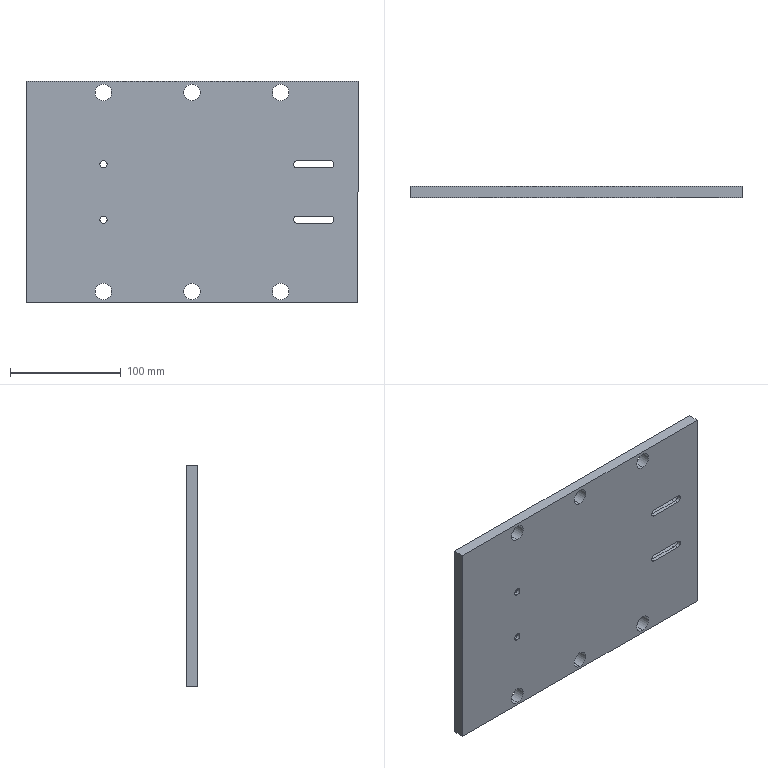Part | SolidWorks | features ICE 3, Extrusion 1, HoleWzd 1, LPattern 1 | 1 solid | 46 faces | box 300 x 10 x 200 mm | volume 580619 mm3 | cylinder 28 | plane 18 | commonest cylinder face diameters 15 x12 6.6 x8 11 x8
STEP:
#1=CARTESIAN_POINT('',(-80.,-1.8,-30.5));
#2=VERTEX_POINT('',#1);
#3=CARTESIAN_POINT('',(-80.,-1.8,-19.5));
#4=VERTEX_POINT('',#3);
#5=CARTESIAN_POINT('',(-80.,-1.8,-25.));
#6=DIRECTION('',(0.,1.,0.));
#7=DIRECTION('',(0.,0.,1.));
#8=AXIS2_PLACEMENT_3D('',#5,#6,#7);
#9=CIRCLE('',#8,5.5);
#10=EDGE_CURVE('',#2,#4,#9,.T.);
#11=ORIENTED_EDGE('',*,*,#10,.F.);
#12=CARTESIAN_POINT('',(-80.,5.,-30.5));
#13=VERTEX_POINT('',#12);
#14=CARTESIAN_POINT('',(-80.,5.,-30.5));
#15=DIRECTION('',(0.,1.,0.));
#16=VECTOR('',#15,1000.);
#17=LINE('',#14,#16);
#18=EDGE_CURVE('',#2,#13,#17,.T.);
#19=ORIENTED_EDGE('',*,*,#18,.T.);
#20=CARTESIAN_POINT('',(-80.,5.,-19.5));
#21=VERTEX_POINT('',#20);
#22=CARTESIAN_POINT('',(-80.,5.,-25.));
#23=DIRECTION('',(0.,1.,0.));
#24=DIRECTION('',(0.,0.,1.));
#25=AXIS2_PLACEMENT_3D('',#22,#23,#24);
#26=CIRCLE('',#25,5.5);
#27=EDGE_CURVE('',#13,#21,#26,.T.);
#28=ORIENTED_EDGE('',*,*,#27,.T.);
#29=CARTESIAN_POINT('',(-80.,5.,-19.5));
#30=DIRECTION('',(0.,1.,0.));
#31=VECTOR('',#30,1000.);
#32=LINE('',#29,#31);
#33=EDGE_CURVE('',#4,#21,#32,.T.);
#34=ORIENTED_EDGE('',*,*,#33,.F.);
#35=EDGE_LOOP('',(#11,#19,#28,#34));
#36=FACE_OUTER_BOUND('',#35,.T.);
#37=CARTESIAN_POINT('',(-80.,5.,-25.));
#38=DIRECTION('',(0.,1.,0.));
#39=DIRECTION('',(0.,0.,1.));
#40=AXIS2_PLACEMENT_3D('',#37,#38,#39);
#41=CYLINDRICAL_SURFACE('',#40,5.5);
#42=ADVANCED_FACE('',(#36),#41,.F.);
#43=CARTESIAN_POINT('',(-80.,-5.,-28.3));
#44=VERTEX_POINT('',#43);
#45=CARTESIAN_POINT('',(-80.,-5.,-21.7));
#46=VERTEX_POINT('',#45);
#47=CARTESIAN_POINT('',(-80.,-5.,-25.));
#48=DIRECTION('',(0.,1.,0.));
#49=DIRECTION('',(0.,0.,1.));
#50=AXIS2_PLACEMENT_3D('',#47,#48,#49);
#51=CIRCLE('',#50,3.3);
#52=EDGE_CURVE('',#44,#46,#51,.T.);
#53=ORIENTED_EDGE('',*,*,#52,.F.);
#54=CARTESIAN_POINT('',(-80.,-1.8,-28.3));
#55=VERTEX_POINT('',#54);
#56=CARTESIAN_POINT('',(-80.,5.,-28.3));
#57=DIRECTION('',(0.,1.,0.));
#58=VECTOR('',#57,1000.);
#59=LINE('',#56,#58);
#60=EDGE_CURVE('',#44,#55,#59,.T.);
#61=ORIENTED_EDGE('',*,*,#60,.T.);
#62=CARTESIAN_POINT('',(-80.,-1.8,-21.7));
#63=VERTEX_POINT('',#62);
#64=CARTESIAN_POINT('',(-80.,-1.8,-25.));
#65=DIRECTION('',(0.,1.,0.));
#66=DIRECTION('',(0.,0.,1.));
#67=AXIS2_PLACEMENT_3D('',#64,#65,#66);
#68=CIRCLE('',#67,3.3);
#69=EDGE_CURVE('',#55,#63,#68,.T.);
#70=ORIENTED_EDGE('',*,*,#69,.T.);
#71=CARTESIAN_POINT('',(-80.,5.,-21.7));
#72=DIRECTION('',(0.,1.,0.));
#73=VECTOR('',#72,1000.);
#74=LINE('',#71,#73);
#75=EDGE_CURVE('',#46,#63,#74,.T.);
#76=ORIENTED_EDGE('',*,*,#75,.F.);
#77=EDGE_LOOP('',(#53,#61,#70,#76));
#78=FACE_OUTER_BOUND('',#77,.T.);
#79=CARTESIAN_POINT('',(-80.,5.,-25.));
#80=DIRECTION('',(0.,1.,0.));
#81=DIRECTION('',(0.,0.,1.));
#82=AXIS2_PLACEMENT_3D('',#79,#80,#81);
#83=CYLINDRICAL_SURFACE('',#82,3.3);
#84=ADVANCED_FACE('',(#78),#83,.F.);
#85=CARTESIAN_POINT('',(-80.,-1.8,19.5));
#86=VERTEX_POINT('',#85);
#87=CARTESIAN_POINT('',(-80.,-1.8,30.5));
#88=VERTEX_POINT('',#87);
#89=CARTESIAN_POINT('',(-80.,-1.8,25.));
#90=DIRECTION('',(0.,1.,0.));
#91=DIRECTION('',(0.,0.,1.));
#92=AXIS2_PLACEMENT_3D('',#89,#90,#91);
#93=CIRCLE('',#92,5.5);
#94=EDGE_CURVE('',#86,#88,#93,.T.);
#95=ORIENTED_EDGE('',*,*,#94,.F.);
#96=CARTESIAN_POINT('',(-80.,5.,19.5));
#97=VERTEX_POINT('',#96);
#98=CARTESIAN_POINT('',(-80.,5.,19.5));
#99=DIRECTION('',(0.,1.,0.));
#100=VECTOR('',#99,1000.);
#101=LINE('',#98,#100);
#102=EDGE_CURVE('',#86,#97,#101,.T.);
#103=ORIENTED_EDGE('',*,*,#102,.T.);
#104=CARTESIAN_POINT('',(-80.,5.,30.5));
#105=VERTEX_POINT('',#104);
#106=CARTESIAN_POINT('',(-80.,5.,25.));
#107=DIRECTION('',(0.,1.,0.));
#108=DIRECTION('',(0.,0.,1.));
#109=AXIS2_PLACEMENT_3D('',#106,#107,#108);
#110=CIRCLE('',#109,5.5);
#111=EDGE_CURVE('',#97,#105,#110,.T.);
#112=ORIENTED_EDGE('',*,*,#111,.T.);
#113=CARTESIAN_POINT('',(-80.,5.,30.5));
#114=DIRECTION('',(0.,1.,0.));
#115=VECTOR('',#114,1000.);
#116=LINE('',#113,#115);
#117=EDGE_CURVE('',#88,#105,#116,.T.);
#118=ORIENTED_EDGE('',*,*,#117,.F.);
#119=EDGE_LOOP('',(#95,#103,#112,#118));
#120=FACE_OUTER_BOUND('',#119,.T.);
#121=CARTESIAN_POINT('',(-80.,5.,25.));
#122=DIRECTION('',(0.,1.,0.));
#123=DIRECTION('',(0.,0.,1.));
#124=AXIS2_PLACEMENT_3D('',#121,#122,#123);
#125=CYLINDRICAL_SURFACE('',#124,5.5);
#126=ADVANCED_FACE('',(#120),#125,.F.);
#127=CARTESIAN_POINT('',(-80.,-5.,21.7));
#128=VERTEX_POINT('',#127);
#129=CARTESIAN_POINT('',(-80.,-5.,28.3));
#130=VERTEX_POINT('',#129);
#131=CARTESIAN_POINT('',(-80.,-5.,25.));
#132=DIRECTION('',(0.,1.,0.));
#133=DIRECTION('',(0.,0.,1.));
#134=AXIS2_PLACEMENT_3D('',#131,#132,#133);
#135=CIRCLE('',#134,3.3);
#136=EDGE_CURVE('',#128,#130,#135,.T.);
#137=ORIENTED_EDGE('',*,*,#136,.F.);
#138=CARTESIAN_POINT('',(-80.,-1.8,21.7));
#139=VERTEX_POINT('',#138);
#140=CARTESIAN_POINT('',(-80.,5.,21.7));
#141=DIRECTION('',(0.,1.,0.));
#142=VECTOR('',#141,1000.);
#143=LINE('',#140,#142);
#144=EDGE_CURVE('',#128,#139,#143,.T.);
#145=ORIENTED_EDGE('',*,*,#144,.T.);
#146=CARTESIAN_POINT('',(-80.,-1.8,28.3));
#147=VERTEX_POINT('',#146);
#148=CARTESIAN_POINT('',(-80.,-1.8,25.));
#149=DIRECTION('',(0.,1.,0.));
#150=DIRECTION('',(0.,0.,1.));
#151=AXIS2_PLACEMENT_3D('',#148,#149,#150);
#152=CIRCLE('',#151,3.3);
#153=EDGE_CURVE('',#139,#147,#152,.T.);
#154=ORIENTED_EDGE('',*,*,#153,.T.);
#155=CARTESIAN_POINT('',(-80.,5.,28.3));
#156=DIRECTION('',(0.,1.,0.));
#157=VECTOR('',#156,1000.);
#158=LINE('',#155,#157);
#159=EDGE_CURVE('',#130,#147,#158,.T.);
#160=ORIENTED_EDGE('',*,*,#159,.F.);
#161=EDGE_LOOP('',(#137,#145,#154,#160));
#162=FACE_OUTER_BOUND('',#161,.T.);
#163=CARTESIAN_POINT('',(-80.,5.,25.));
#164=DIRECTION('',(0.,1.,0.));
#165=DIRECTION('',(0.,0.,1.));
#166=AXIS2_PLACEMENT_3D('',#163,#164,#165);
#167=CYLINDRICAL_SURFACE('',#166,3.3);
#168=ADVANCED_FACE('',(#162),#167,.F.);
#169=CARTESIAN_POINT('',(80.,-5.,82.5));
#170=VERTEX_POINT('',#169);
#171=CARTESIAN_POINT('',(80.,-5.,97.5));
#172=VERTEX_POINT('',#171);
#173=CARTESIAN_POINT('',(80.,-5.,90.));
#174=DIRECTION('',(0.,1.,0.));
#175=DIRECTION('',(0.,0.,1.));
#176=AXIS2_PLACEMENT_3D('',#173,#174,#175);
#177=CIRCLE('',#176,7.5);
#178=EDGE_CURVE('',#170,#172,#177,.T.);
#179=ORIENTED_EDGE('',*,*,#178,.F.);
#180=CARTESIAN_POINT('',(80.,5.,82.5));
#181=VERTEX_POINT('',#180);
#182=CARTESIAN_POINT('',(80.,-5.,82.5));
#183=DIRECTION('',(0.,1.,0.));
#184=VECTOR('',#183,1000.);
#185=LINE('',#182,#184);
#186=EDGE_CURVE('',#170,#181,#185,.T.);
#187=ORIENTED_EDGE('',*,*,#186,.T.);
#188=CARTESIAN_POINT('',(80.,5.,97.5));
#189=VERTEX_POINT('',#188);
#190=CARTESIAN_POINT('',(80.,5.,90.));
#191=DIRECTION('',(0.,1.,0.));
#192=DIRECTION('',(0.,0.,1.));
#193=AXIS2_PLACEMENT_3D('',#190,#191,#192);
#194=CIRCLE('',#193,7.5);
#195=EDGE_CURVE('',#181,#189,#194,.T.);
#196=ORIENTED_EDGE('',*,*,#195,.T.);
#197=CARTESIAN_POINT('',(80.,-5.,97.5));
#198=DIRECTION('',(0.,1.,0.));
#199=VECTOR('',#198,1000.);
#200=LINE('',#197,#199);
#201=EDGE_CURVE('',#172,#189,#200,.T.);
#202=ORIENTED_EDGE('',*,*,#201,.F.);
#203=EDGE_LOOP('',(#179,#187,#196,#202));
#204=FACE_OUTER_BOUND('',#203,.T.);
#205=CARTESIAN_POINT('',(80.,-5.,90.));
#206=DIRECTION('',(0.,1.,0.));
#207=DIRECTION('',(0.,0.,1.));
#208=AXIS2_PLACEMENT_3D('',#205,#206,#207);
#209=CYLINDRICAL_SURFACE('',#208,7.5);
#210=ADVANCED_FACE('',(#204),#209,.F.);
#211=CARTESIAN_POINT('',(80.,-5.,-97.5));
#212=VERTEX_POINT('',#211);
#213=CARTESIAN_POINT('',(80.,-5.,-82.5));
#214=VERTEX_POINT('',#213);
#215=CARTESIAN_POINT('',(80.,-5.,-90.));
#216=DIRECTION('',(0.,1.,0.));
#217=DIRECTION('',(0.,0.,1.));
#218=AXIS2_PLACEMENT_3D('',#215,#216,#217);
#219=CIRCLE('',#218,7.5);
#220=EDGE_CURVE('',#212,#214,#219,.T.);
#221=ORIENTED_EDGE('',*,*,#220,.F.);
#222=CARTESIAN_POINT('',(80.,5.,-97.5));
#223=VERTEX_POINT('',#222);
#224=CARTESIAN_POINT('',(80.,-5.,-97.5));
#225=DIRECTION('',(0.,1.,0.));
#226=VECTOR('',#225,1000.);
#227=LINE('',#224,#226);
#228=EDGE_CURVE('',#212,#223,#227,.T.);
#229=ORIENTED_EDGE('',*,*,#228,.T.);
#230=CARTESIAN_POINT('',(80.,5.,-82.5));
#231=VERTEX_POINT('',#230);
#232=CARTESIAN_POINT('',(80.,5.,-90.));
#233=DIRECTION('',(0.,1.,0.));
#234=DIRECTION('',(0.,0.,1.));
#235=AXIS2_PLACEMENT_3D('',#232,#233,#234);
#236=CIRCLE('',#235,7.5);
#237=EDGE_CURVE('',#223,#231,#236,.T.);
#238=ORIENTED_EDGE('',*,*,#237,.T.);
#239=CARTESIAN_POINT('',(80.,-5.,-82.5));
#240=DIRECTION('',(0.,1.,0.));
#241=VECTOR('',#240,1000.);
#242=LINE('',#239,#241);
#243=EDGE_CURVE('',#214,#231,#242,.T.);
#244=ORIENTED_EDGE('',*,*,#243,.F.);
#245=EDGE_LOOP('',(#221,#229,#238,#244));
#246=FACE_OUTER_BOUND('',#245,.T.);
#247=CARTESIAN_POINT('',(80.,-5.,-90.));
#248=DIRECTION('',(0.,1.,0.));
#249=DIRECTION('',(0.,0.,1.));
#250=AXIS2_PLACEMENT_3D('',#247,#248,#249);
#251=CYLINDRICAL_SURFACE('',#250,7.5);
#252=ADVANCED_FACE('',(#246),#251,.F.);
#253=CARTESIAN_POINT('',(0.,-5.,-97.5));
#254=VERTEX_POINT('',#253);
#255=CARTESIAN_POINT('',(0.,-5.,-82.5));
#256=VERTEX_POINT('',#255);
#257=CARTESIAN_POINT('',(0.,-5.,-90.));
#258=DIRECTION('',(0.,1.,0.));
#259=DIRECTION('',(0.,0.,1.));
#260=AXIS2_PLACEMENT_3D('',#257,#258,#259);
#261=CIRCLE('',#260,7.5);
#262=EDGE_CURVE('',#254,#256,#261,.T.);
#263=ORIENTED_EDGE('',*,*,#262,.F.);
#264=CARTESIAN_POINT('',(0.,5.,-97.5));
#265=VERTEX_POINT('',#264);
#266=CARTESIAN_POINT('',(0.,-5.,-97.5));
#267=DIRECTION('',(0.,1.,0.));
#268=VECTOR('',#267,1000.);
#269=LINE('',#266,#268);
#270=EDGE_CURVE('',#254,#265,#269,.T.);
#271=ORIENTED_EDGE('',*,*,#270,.T.);
#272=CARTESIAN_POINT('',(0.,5.,-82.5));
#273=VERTEX_POINT('',#272);
#274=CARTESIAN_POINT('',(0.,5.,-90.));
#275=DIRECTION('',(0.,1.,0.));
#276=DIRECTION('',(0.,0.,1.));
#277=AXIS2_PLACEMENT_3D('',#274,#275,#276);
#278=CIRCLE('',#277,7.5);
#279=EDGE_CURVE('',#265,#273,#278,.T.);
#280=ORIENTED_EDGE('',*,*,#279,.T.);
#281=CARTESIAN_POINT('',(0.,-5.,-82.5));
#282=DIRECTION('',(0.,1.,0.));
#283=VECTOR('',#282,1000.);
#284=LINE('',#281,#283);
#285=EDGE_CURVE('',#256,#273,#284,.T.);
#286=ORIENTED_EDGE('',*,*,#285,.F.);
#287=EDGE_LOOP('',(#263,#271,#280,#286));
#288=FACE_OUTER_BOUND('',#287,.T.);
#289=CARTESIAN_POINT('',(0.,-5.,-90.));
#290=DIRECTION('',(0.,1.,0.));
#291=DIRECTION('',(0.,0.,1.));
#292=AXIS2_PLACEMENT_3D('',#289,#290,#291);
#293=CYLINDRICAL_SURFACE('',#292,7.5);
#294=ADVANCED_FACE('',(#288),#293,.F.);
#295=CARTESIAN_POINT('',(0.,-5.,82.5));
#296=VERTEX_POINT('',#295);
#297=CARTESIAN_POINT('',(0.,-5.,97.5));
#298=VERTEX_POINT('',#297);
#299=CARTESIAN_POINT('',(0.,-5.,90.));
#300=DIRECTION('',(0.,1.,0.));
#301=DIRECTION('',(0.,0.,1.));
#302=AXIS2_PLACEMENT_3D('',#299,#300,#301);
#303=CIRCLE('',#302,7.5);
#304=EDGE_CURVE('',#296,#298,#303,.T.);
#305=ORIENTED_EDGE('',*,*,#304,.F.);
#306=CARTESIAN_POINT('',(0.,5.,82.5));
#307=VERTEX_POINT('',#306);
#308=CARTESIAN_POINT('',(0.,-5.,82.5));
#309=DIRECTION('',(0.,1.,0.));
#310=VECTOR('',#309,1000.);
#311=LINE('',#308,#310);
#312=EDGE_CURVE('',#296,#307,#311,.T.);
#313=ORIENTED_EDGE('',*,*,#312,.T.);
#314=CARTESIAN_POINT('',(0.,5.,97.5));
#315=VERTEX_POINT('',#314);
#316=CARTESIAN_POINT('',(0.,5.,90.));
#317=DIRECTION('',(0.,1.,0.));
#318=DIRECTION('',(0.,0.,1.));
#319=AXIS2_PLACEMENT_3D('',#316,#317,#318);
#320=CIRCLE('',#319,7.5);
#321=EDGE_CURVE('',#307,#315,#320,.T.);
#322=ORIENTED_EDGE('',*,*,#321,.T.);
#323=CARTESIAN_POINT('',(0.,-5.,97.5));
#324=DIRECTION('',(0.,1.,0.));
#325=VECTOR('',#324,1000.);
#326=LINE('',#323,#325);
#327=EDGE_CURVE('',#298,#315,#326,.T.);
#328=ORIENTED_EDGE('',*,*,#327,.F.);
#329=EDGE_LOOP('',(#305,#313,#322,#328));
#330=FACE_OUTER_BOUND('',#329,.T.);
#331=CARTESIAN_POINT('',(0.,-5.,90.));
#332=DIRECTION('',(0.,1.,0.));
#333=DIRECTION('',(0.,0.,1.));
#334=AXIS2_PLACEMENT_3D('',#331,#332,#333);
#335=CYLINDRICAL_SURFACE('',#334,7.5);
#336=ADVANCED_FACE('',(#330),#335,.F.);
#337=CARTESIAN_POINT('',(-80.,-5.,-97.5));
#338=VERTEX_POINT('',#337);
#339=CARTESIAN_POINT('',(-80.,-5.,-82.5));
#340=VERTEX_POINT('',#339);
#341=CARTESIAN_POINT('',(-80.,-5.,-90.));
#342=DIRECTION('',(0.,1.,0.));
#343=DIRECTION('',(0.,0.,1.));
#344=AXIS2_PLACEMENT_3D('',#341,#342,#343);
#345=CIRCLE('',#344,7.5);
#346=EDGE_CURVE('',#338,#340,#345,.T.);
#347=ORIENTED_EDGE('',*,*,#346,.F.);
#348=CARTESIAN_POINT('',(-80.,5.,-97.5));
#349=VERTEX_POINT('',#348);
#350=CARTESIAN_POINT('',(-80.,-5.,-97.5));
#351=DIRECTION('',(0.,1.,0.));
#352=VECTOR('',#351,1000.);
#353=LINE('',#350,#352);
#354=EDGE_CURVE('',#338,#349,#353,.T.);
#355=ORIENTED_EDGE('',*,*,#354,.T.);
#356=CARTESIAN_POINT('',(-80.,5.,-82.5));
#357=VERTEX_POINT('',#356);
#358=CARTESIAN_POINT('',(-80.,5.,-90.));
#359=DIRECTION('',(0.,1.,0.));
#360=DIRECTION('',(0.,0.,1.));
#361=AXIS2_PLACEMENT_3D('',#358,#359,#360);
#362=CIRCLE('',#361,7.5);
#363=EDGE_CURVE('',#349,#357,#362,.T.);
#364=ORIENTED_EDGE('',*,*,#363,.T.);
#365=CARTESIAN_POINT('',(-80.,-5.,-82.5));
#366=DIRECTION('',(0.,1.,0.));
#367=VECTOR('',#366,1000.);
#368=LINE('',#365,#367);
#369=EDGE_CURVE('',#340,#357,#368,.T.);
#370=ORIENTED_EDGE('',*,*,#369,.F.);
#371=EDGE_LOOP('',(#347,#355,#364,#370));
#372=FACE_OUTER_BOUND('',#371,.T.);
#373=CARTESIAN_POINT('',(-80.,-5.,-90.));
#374=DIRECTION('',(0.,1.,0.));
#375=DIRECTION('',(0.,0.,1.));
#376=AXIS2_PLACEMENT_3D('',#373,#374,#375);
#377=CYLINDRICAL_SURFACE('',#376,7.5);
#378=ADVANCED_FACE('',(#372),#377,.F.);
#379=CARTESIAN_POINT('',(-80.,-5.,82.5));
#380=VERTEX_POINT('',#379);
#381=CARTESIAN_POINT('',(-80.,-5.,97.5));
#382=VERTEX_POINT('',#381);
#383=CARTESIAN_POINT('',(-80.,-5.,90.));
#384=DIRECTION('',(0.,1.,0.));
#385=DIRECTION('',(0.,0.,1.));
#386=AXIS2_PLACEMENT_3D('',#383,#384,#385);
#387=CIRCLE('',#386,7.5);
#388=EDGE_CURVE('',#380,#382,#387,.T.);
#389=ORIENTED_EDGE('',*,*,#388,.F.);
#390=CARTESIAN_POINT('',(-80.,5.,82.5));
#391=VERTEX_POINT('',#390);
#392=CARTESIAN_POINT('',(-80.,-5.,82.5));
#393=DIRECTION('',(0.,1.,0.));
#394=VECTOR('',#393,1000.);
#395=LINE('',#392,#394);
#396=EDGE_CURVE('',#380,#391,#395,.T.);
#397=ORIENTED_EDGE('',*,*,#396,.T.);
#398=CARTESIAN_POINT('',(-80.,5.,97.5));
#399=VERTEX_POINT('',#398);
#400=CARTESIAN_POINT('',(-80.,5.,90.));
#401=DIRECTION('',(0.,1.,0.));
#402=DIRECTION('',(0.,0.,1.));
#403=AXIS2_PLACEMENT_3D('',#400,#401,#402);
#404=CIRCLE('',#403,7.5);
#405=EDGE_CURVE('',#391,#399,#404,.T.);
#406=ORIENTED_EDGE('',*,*,#405,.T.);
#407=CARTESIAN_POINT('',(-80.,-5.,97.5));
#408=DIRECTION('',(0.,1.,0.));
#409=VECTOR('',#408,1000.);
#410=LINE('',#407,#409);
#411=EDGE_CURVE('',#382,#399,#410,.T.);
#412=ORIENTED_EDGE('',*,*,#411,.F.);
#413=EDGE_LOOP('',(#389,#397,#406,#412));
#414=FACE_OUTER_BOUND('',#413,.T.);
#415=CARTESIAN_POINT('',(-80.,-5.,90.));
#416=DIRECTION('',(0.,1.,0.));
#417=DIRECTION('',(0.,0.,1.));
#418=AXIS2_PLACEMENT_3D('',#415,#416,#417);
#419=CYLINDRICAL_SURFACE('',#418,7.5);
#420=ADVANCED_FACE('',(#414),#419,.F.);
#421=CARTESIAN_POINT('',(125.,-1.8,21.7));
#422=VERTEX_POINT('',#421);
#423=CARTESIAN_POINT('',(125.,-1.8,28.3));
#424=VERTEX_POINT('',#423);
#425=CARTESIAN_POINT('',(125.,-1.8,25.));
#426=DIRECTION('',(0.,-1.,0.));
#427=DIRECTION('',(0.,0.,1.));
#428=AXIS2_PLACEMENT_3D('',#425,#426,#427);
#429=CIRCLE('',#428,3.3);
#430=EDGE_CURVE('',#422,#424,#429,.T.);
#431=ORIENTED_EDGE('',*,*,#430,.F.);
#432=CARTESIAN_POINT('',(125.,-5.,21.7));
#433=VERTEX_POINT('',#432);
#434=CARTESIAN_POINT('',(125.,-5.,21.7));
#435=DIRECTION('',(0.,1.,0.));
#436=VECTOR('',#435,1000.);
#437=LINE('',#434,#436);
#438=EDGE_CURVE('',#433,#422,#437,.T.);
#439=ORIENTED_EDGE('',*,*,#438,.F.);
#440=CARTESIAN_POINT('',(125.,-5.,28.3));
#441=VERTEX_POINT('',#440);
#442=CARTESIAN_POINT('',(125.,-5.,25.));
#443=DIRECTION('',(0.,1.,0.));
#444=DIRECTION('',(0.,0.,1.));
#445=AXIS2_PLACEMENT_3D('',#442,#443,#444);
#446=CIRCLE('',#445,3.3);
#447=EDGE_CURVE('',#441,#433,#446,.T.);
#448=ORIENTED_EDGE('',*,*,#447,.F.);
#449=CARTESIAN_POINT('',(125.,-5.,28.3));
#450=DIRECTION('',(0.,1.,0.));
#451=VECTOR('',#450,1000.);
#452=LINE('',#449,#451);
#453=EDGE_CURVE('',#441,#424,#452,.T.);
#454=ORIENTED_EDGE('',*,*,#453,.T.);
#455=EDGE_LOOP('',(#431,#439,#448,#454));
#456=FACE_OUTER_BOUND('',#455,.T.);
#457=CARTESIAN_POINT('',(125.,-5.,25.));
#458=DIRECTION('',(0.,1.,0.));
#459=DIRECTION('',(0.,0.,1.));
#460=AXIS2_PLACEMENT_3D('',#457,#458,#459);
#461=CYLINDRICAL_SURFACE('',#460,3.3);
#462=ADVANCED_FACE('',(#456),#461,.F.);
#463=CARTESIAN_POINT('',(95.,-1.8,28.3));
#464=VERTEX_POINT('',#463);
#465=CARTESIAN_POINT('',(125.,-1.8,28.3));
#466=DIRECTION('',(-1.,0.,0.));
#467=VECTOR('',#466,1000.);
#468=LINE('',#465,#467);
#469=EDGE_CURVE('',#424,#464,#468,.T.);
#470=ORIENTED_EDGE('',*,*,#469,.F.);
#471=ORIENTED_EDGE('',*,*,#453,.F.);
#472=CARTESIAN_POINT('',(95.,-5.,28.3));
#473=VERTEX_POINT('',#472);
#474=CARTESIAN_POINT('',(125.,-5.,28.3));
#475=DIRECTION('',(1.,0.,0.));
#476=VECTOR('',#475,1000.);
#477=LINE('',#474,#476);
#478=EDGE_CURVE('',#473,#441,#477,.T.);
#479=ORIENTED_EDGE('',*,*,#478,.F.);
#480=CARTESIAN_POINT('',(95.,-5.,28.3));
#481=DIRECTION('',(0.,1.,0.));
#482=VECTOR('',#481,1000.);
#483=LINE('',#480,#482);
#484=EDGE_CURVE('',#473,#464,#483,.T.);
#485=ORIENTED_EDGE('',*,*,#484,.T.);
#486=EDGE_LOOP('',(#470,#471,#479,#485));
#487=FACE_OUTER_BOUND('',#486,.T.);
#488=CARTESIAN_POINT('',(125.,-5.,28.3));
#489=DIRECTION('',(0.,0.,1.));
#490=DIRECTION('',(1.,0.,0.));
#491=AXIS2_PLACEMENT_3D('',#488,#489,#490);
#492=PLANE('',#491);
#493=ADVANCED_FACE('',(#487),#492,.F.);
#494=CARTESIAN_POINT('',(95.,-1.8,21.7));
#495=VERTEX_POINT('',#494);
#496=CARTESIAN_POINT('',(95.,-1.8,25.));
#497=DIRECTION('',(0.,-1.,0.));
#498=DIRECTION('',(0.,0.,1.));
#499=AXIS2_PLACEMENT_3D('',#496,#497,#498);
#500=CIRCLE('',#499,3.3);
#501=EDGE_CURVE('',#464,#495,#500,.T.);
#502=ORIENTED_EDGE('',*,*,#501,.F.);
#503=ORIENTED_EDGE('',*,*,#484,.F.);
#504=CARTESIAN_POINT('',(95.,-5.,21.7));
#505=VERTEX_POINT('',#504);
#506=CARTESIAN_POINT('',(95.,-5.,25.));
#507=DIRECTION('',(0.,1.,0.));
#508=DIRECTION('',(0.,0.,1.));
#509=AXIS2_PLACEMENT_3D('',#506,#507,#508);
#510=CIRCLE('',#509,3.3);
#511=EDGE_CURVE('',#505,#473,#510,.T.);
#512=ORIENTED_EDGE('',*,*,#511,.F.);
#513=CARTESIAN_POINT('',(95.,-5.,21.7));
#514=DIRECTION('',(0.,1.,0.));
#515=VECTOR('',#514,1000.);
#516=LINE('',#513,#515);
#517=EDGE_CURVE('',#505,#495,#516,.T.);
#518=ORIENTED_EDGE('',*,*,#517,.T.);
#519=EDGE_LOOP('',(#502,#503,#512,#518));
#520=FACE_OUTER_BOUND('',#519,.T.);
#521=CARTESIAN_POINT('',(95.,-5.,25.));
#522=DIRECTION('',(0.,1.,0.));
#523=DIRECTION('',(0.,0.,1.));
#524=AXIS2_PLACEMENT_3D('',#521,#522,#523);
#525=CYLINDRICAL_SURFACE('',#524,3.3);
#526=ADVANCED_FACE('',(#520),#525,.F.);
#527=CARTESIAN_POINT('',(125.,-1.8,21.7));
#528=DIRECTION('',(1.,0.,0.));
#529=VECTOR('',#528,1000.);
#530=LINE('',#527,#529);
#531=EDGE_CURVE('',#495,#422,#530,.T.);
#532=ORIENTED_EDGE('',*,*,#531,.F.);
#533=ORIENTED_EDGE('',*,*,#517,.F.);
#534=CARTESIAN_POINT('',(125.,-5.,21.7));
#535=DIRECTION('',(-1.,0.,0.));
#536=VECTOR('',#535,1000.);
#537=LINE('',#534,#536);
#538=EDGE_CURVE('',#433,#505,#537,.T.);
#539=ORIENTED_EDGE('',*,*,#538,.F.);
#540=ORIENTED_EDGE('',*,*,#438,.T.);
#541=EDGE_LOOP('',(#532,#533,#539,#540));
#542=FACE_OUTER_BOUND('',#541,.T.);
#543=CARTESIAN_POINT('',(125.,-5.,21.7));
#544=DIRECTION('',(0.,0.,-1.));
#545=DIRECTION('',(-1.,0.,0.));
#546=AXIS2_PLACEMENT_3D('',#543,#544,#545);
#547=PLANE('',#546);
#548=ADVANCED_FACE('',(#542),#547,.F.);
#549=CARTESIAN_POINT('',(125.,-1.8,-28.3));
#550=VERTEX_POINT('',#549);
#551=CARTESIAN_POINT('',(125.,-1.8,-21.7));
#552=VERTEX_POINT('',#551);
#553=CARTESIAN_POINT('',(125.,-1.8,-25.));
#554=DIRECTION('',(0.,-1.,0.));
#555=DIRECTION('',(0.,0.,1.));
#556=AXIS2_PLACEMENT_3D('',#553,#554,#555);
#557=CIRCLE('',#556,3.3);
#558=EDGE_CURVE('',#550,#552,#557,.T.);
#559=ORIENTED_EDGE('',*,*,#558,.F.);
#560=CARTESIAN_POINT('',(125.,-5.,-28.3));
#561=VERTEX_POINT('',#560);
#562=CARTESIAN_POINT('',(125.,-5.,-28.3));
#563=DIRECTION('',(0.,1.,0.));
#564=VECTOR('',#563,1000.);
#565=LINE('',#562,#564);
#566=EDGE_CURVE('',#561,#550,#565,.T.);
#567=ORIENTED_EDGE('',*,*,#566,.F.);
#568=CARTESIAN_POINT('',(125.,-5.,-21.7));
#569=VERTEX_POINT('',#568);
#570=CARTESIAN_POINT('',(125.,-5.,-25.));
#571=DIRECTION('',(0.,1.,0.));
#572=DIRECTION('',(0.,0.,1.));
#573=AXIS2_PLACEMENT_3D('',#570,#571,#572);
#574=CIRCLE('',#573,3.3);
#575=EDGE_CURVE('',#569,#561,#574,.T.);
#576=ORIENTED_EDGE('',*,*,#575,.F.);
#577=CARTESIAN_POINT('',(125.,-5.,-21.7));
#578=DIRECTION('',(0.,1.,0.));
#579=VECTOR('',#578,1000.);
#580=LINE('',#577,#579);
#581=EDGE_CURVE('',#569,#552,#580,.T.);
#582=ORIENTED_EDGE('',*,*,#581,.T.);
#583=EDGE_LOOP('',(#559,#567,#576,#582));
#584=FACE_OUTER_BOUND('',#583,.T.);
#585=CARTESIAN_POINT('',(125.,-5.,-25.));
#586=DIRECTION('',(0.,1.,0.));
#587=DIRECTION('',(0.,0.,1.));
#588=AXIS2_PLACEMENT_3D('',#585,#586,#587);
#589=CYLINDRICAL_SURFACE('',#588,3.3);
#590=ADVANCED_FACE('',(#584),#589,.F.);
#591=CARTESIAN_POINT('',(95.,-1.8,-21.7));
#592=VERTEX_POINT('',#591);
#593=CARTESIAN_POINT('',(125.,-1.8,-21.7));
#594=DIRECTION('',(-1.,0.,0.));
#595=VECTOR('',#594,1000.);
#596=LINE('',#593,#595);
#597=EDGE_CURVE('',#552,#592,#596,.T.);
#598=ORIENTED_EDGE('',*,*,#597,.F.);
#599=ORIENTED_EDGE('',*,*,#581,.F.);
#600=CARTESIAN_POINT('',(95.,-5.,-21.7));
#601=VERTEX_POINT('',#600);
#602=CARTESIAN_POINT('',(125.,-5.,-21.7));
#603=DIRECTION('',(1.,0.,0.));
#604=VECTOR('',#603,1000.);
#605=LINE('',#602,#604);
#606=EDGE_CURVE('',#601,#569,#605,.T.);
#607=ORIENTED_EDGE('',*,*,#606,.F.);
#608=CARTESIAN_POINT('',(95.,-5.,-21.7));
#609=DIRECTION('',(0.,1.,0.));
#610=VECTOR('',#609,1000.);
#611=LINE('',#608,#610);
#612=EDGE_CURVE('',#601,#592,#611,.T.);
#613=ORIENTED_EDGE('',*,*,#612,.T.);
#614=EDGE_LOOP('',(#598,#599,#607,#613));
#615=FACE_OUTER_BOUND('',#614,.T.);
#616=CARTESIAN_POINT('',(125.,-5.,-21.7));
#617=DIRECTION('',(0.,0.,1.));
#618=DIRECTION('',(1.,0.,0.));
#619=AXIS2_PLACEMENT_3D('',#616,#617,#618);
#620=PLANE('',#619);
#621=ADVANCED_FACE('',(#615),#620,.F.);
#622=CARTESIAN_POINT('',(95.,-1.8,-28.3));
#623=VERTEX_POINT('',#622);
#624=CARTESIAN_POINT('',(95.,-1.8,-25.));
#625=DIRECTION('',(0.,-1.,0.));
#626=DIRECTION('',(0.,0.,1.));
#627=AXIS2_PLACEMENT_3D('',#624,#625,#626);
#628=CIRCLE('',#627,3.3);
#629=EDGE_CURVE('',#592,#623,#628,.T.);
#630=ORIENTED_EDGE('',*,*,#629,.F.);
#631=ORIENTED_EDGE('',*,*,#612,.F.);
#632=CARTESIAN_POINT('',(95.,-5.,-28.3));
#633=VERTEX_POINT('',#632);
#634=CARTESIAN_POINT('',(95.,-5.,-25.));
#635=DIRECTION('',(0.,1.,0.));
#636=DIRECTION('',(0.,0.,1.));
#637=AXIS2_PLACEMENT_3D('',#634,#635,#636);
#638=CIRCLE('',#637,3.3);
#639=EDGE_CURVE('',#633,#601,#638,.T.);
#640=ORIENTED_EDGE('',*,*,#639,.F.);
#641=CARTESIAN_POINT('',(95.,-5.,-28.3));
#642=DIRECTION('',(0.,1.,0.));
#643=VECTOR('',#642,1000.);
#644=LINE('',#641,#643);
#645=EDGE_CURVE('',#633,#623,#644,.T.);
#646=ORIENTED_EDGE('',*,*,#645,.T.);
#647=EDGE_LOOP('',(#630,#631,#640,#646));
#648=FACE_OUTER_BOUND('',#647,.T.);
#649=CARTESIAN_POINT('',(95.,-5.,-25.));
#650=DIRECTION('',(0.,1.,0.));
#651=DIRECTION('',(0.,0.,1.));
#652=AXIS2_PLACEMENT_3D('',#649,#650,#651);
#653=CYLINDRICAL_SURFACE('',#652,3.3);
#654=ADVANCED_FACE('',(#648),#653,.F.);
#655=CARTESIAN_POINT('',(125.,-1.8,-28.3));
#656=DIRECTION('',(1.,0.,0.));
#657=VECTOR('',#656,1000.);
#658=LINE('',#655,#657);
#659=EDGE_CURVE('',#623,#550,#658,.T.);
#660=ORIENTED_EDGE('',*,*,#659,.F.);
#661=ORIENTED_EDGE('',*,*,#645,.F.);
#662=CARTESIAN_POINT('',(125.,-5.,-28.3));
#663=DIRECTION('',(-1.,0.,0.));
#664=VECTOR('',#663,1000.);
#665=LINE('',#662,#664);
#666=EDGE_CURVE('',#561,#633,#665,.T.);
#667=ORIENTED_EDGE('',*,*,#666,.F.);
#668=ORIENTED_EDGE('',*,*,#566,.T.);
#669=EDGE_LOOP('',(#660,#661,#667,#668));
#670=FACE_OUTER_BOUND('',#669,.T.);
#671=CARTESIAN_POINT('',(125.,-5.,-28.3));
#672=DIRECTION('',(0.,0.,-1.));
#673=DIRECTION('',(-1.,0.,0.));
#674=AXIS2_PLACEMENT_3D('',#671,#672,#673);
#675=PLANE('',#674);
#676=ADVANCED_FACE('',(#670),#675,.F.);
#677=ORIENTED_EDGE('',*,*,#396,.F.);
#678=CARTESIAN_POINT('',(-80.,-5.,90.));
#679=DIRECTION('',(0.,1.,0.));
#680=DIRECTION('',(0.,0.,1.));
#681=AXIS2_PLACEMENT_3D('',#678,#679,#680);
#682=CIRCLE('',#681,7.5);
#683=EDGE_CURVE('',#382,#380,#682,.T.);
#684=ORIENTED_EDGE('',*,*,#683,.F.);
#685=ORIENTED_EDGE('',*,*,#411,.T.);
#686=CARTESIAN_POINT('',(-80.,5.,90.));
#687=DIRECTION('',(0.,1.,0.));
#688=DIRECTION('',(0.,0.,1.));
#689=AXIS2_PLACEMENT_3D('',#686,#687,#688);
#690=CIRCLE('',#689,7.5);
#691=EDGE_CURVE('',#399,#391,#690,.T.);
#692=ORIENTED_EDGE('',*,*,#691,.T.);
#693=EDGE_LOOP('',(#677,#684,#685,#692));
#694=FACE_OUTER_BOUND('',#693,.T.);
#695=CARTESIAN_POINT('',(-80.,-5.,90.));
#696=DIRECTION('',(0.,1.,0.));
#697=DIRECTION('',(0.,0.,1.));
#698=AXIS2_PLACEMENT_3D('',#695,#696,#697);
#699=CYLINDRICAL_SURFACE('',#698,7.5);
#700=ADVANCED_FACE('',(#694),#699,.F.);
#701=ORIENTED_EDGE('',*,*,#354,.F.);
#702=CARTESIAN_POINT('',(-80.,-5.,-90.));
#703=DIRECTION('',(0.,1.,0.));
#704=DIRECTION('',(0.,0.,1.));
#705=AXIS2_PLACEMENT_3D('',#702,#703,#704);
#706=CIRCLE('',#705,7.5);
#707=EDGE_CURVE('',#340,#338,#706,.T.);
#708=ORIENTED_EDGE('',*,*,#707,.F.);
#709=ORIENTED_EDGE('',*,*,#369,.T.);
#710=CARTESIAN_POINT('',(-80.,5.,-90.));
#711=DIRECTION('',(0.,1.,0.));
#712=DIRECTION('',(0.,0.,1.));
#713=AXIS2_PLACEMENT_3D('',#710,#711,#712);
#714=CIRCLE('',#713,7.5);
#715=EDGE_CURVE('',#357,#349,#714,.T.);
#716=ORIENTED_EDGE('',*,*,#715,.T.);
#717=EDGE_LOOP('',(#701,#708,#709,#716));
#718=FACE_OUTER_BOUND('',#717,.T.);
#719=CARTESIAN_POINT('',(-80.,-5.,-90.));
#720=DIRECTION('',(0.,1.,0.));
#721=DIRECTION('',(0.,0.,1.));
#722=AXIS2_PLACEMENT_3D('',#719,#720,#721);
#723=CYLINDRICAL_SURFACE('',#722,7.5);
#724=ADVANCED_FACE('',(#718),#723,.F.);
#725=ORIENTED_EDGE('',*,*,#312,.F.);
#726=CARTESIAN_POINT('',(0.,-5.,90.));
#727=DIRECTION('',(0.,1.,0.));
#728=DIRECTION('',(0.,0.,1.));
#729=AXIS2_PLACEMENT_3D('',#726,#727,#728);
#730=CIRCLE('',#729,7.5);
#731=EDGE_CURVE('',#298,#296,#730,.T.);
#732=ORIENTED_EDGE('',*,*,#731,.F.);
#733=ORIENTED_EDGE('',*,*,#327,.T.);
#734=CARTESIAN_POINT('',(0.,5.,90.));
#735=DIRECTION('',(0.,1.,0.));
#736=DIRECTION('',(0.,0.,1.));
#737=AXIS2_PLACEMENT_3D('',#734,#735,#736);
#738=CIRCLE('',#737,7.5);
#739=EDGE_CURVE('',#315,#307,#738,.T.);
#740=ORIENTED_EDGE('',*,*,#739,.T.);
#741=EDGE_LOOP('',(#725,#732,#733,#740));
#742=FACE_OUTER_BOUND('',#741,.T.);
#743=CARTESIAN_POINT('',(0.,-5.,90.));
#744=DIRECTION('',(0.,1.,0.));
#745=DIRECTION('',(0.,0.,1.));
#746=AXIS2_PLACEMENT_3D('',#743,#744,#745);
#747=CYLINDRICAL_SURFACE('',#746,7.5);
#748=ADVANCED_FACE('',(#742),#747,.F.);
#749=ORIENTED_EDGE('',*,*,#270,.F.);
#750=CARTESIAN_POINT('',(0.,-5.,-90.));
#751=DIRECTION('',(0.,1.,0.));
#752=DIRECTION('',(0.,0.,1.));
#753=AXIS2_PLACEMENT_3D('',#750,#751,#752);
#754=CIRCLE('',#753,7.5);
#755=EDGE_CURVE('',#256,#254,#754,.T.);
#756=ORIENTED_EDGE('',*,*,#755,.F.);
#757=ORIENTED_EDGE('',*,*,#285,.T.);
#758=CARTESIAN_POINT('',(0.,5.,-90.));
#759=DIRECTION('',(0.,1.,0.));
#760=DIRECTION('',(0.,0.,1.));
#761=AXIS2_PLACEMENT_3D('',#758,#759,#760);
#762=CIRCLE('',#761,7.5);
#763=EDGE_CURVE('',#273,#265,#762,.T.);
#764=ORIENTED_EDGE('',*,*,#763,.T.);
#765=EDGE_LOOP('',(#749,#756,#757,#764));
#766=FACE_OUTER_BOUND('',#765,.T.);
#767=CARTESIAN_POINT('',(0.,-5.,-90.));
#768=DIRECTION('',(0.,1.,0.));
#769=DIRECTION('',(0.,0.,1.));
#770=AXIS2_PLACEMENT_3D('',#767,#768,#769);
#771=CYLINDRICAL_SURFACE('',#770,7.5);
#772=ADVANCED_FACE('',(#766),#771,.F.);
#773=CARTESIAN_POINT('',(150.,-5.,100.));
#774=VERTEX_POINT('',#773);
#775=CARTESIAN_POINT('',(150.,-5.,-100.));
#776=VERTEX_POINT('',#775);
#777=CARTESIAN_POINT('',(150.,-5.,-100.));
#778=DIRECTION('',(0.,0.,-1.));
#779=VECTOR('',#778,1000.);
#780=LINE('',#777,#779);
#781=EDGE_CURVE('',#774,#776,#780,.T.);
#782=ORIENTED_EDGE('',*,*,#781,.T.);
#783=CARTESIAN_POINT('',(150.,5.,-100.));
#784=VERTEX_POINT('',#783);
#785=CARTESIAN_POINT('',(150.,5.,-100.));
#786=DIRECTION('',(0.,-1.,0.));
#787=VECTOR('',#786,1000.);
#788=LINE('',#785,#787);
#789=EDGE_CURVE('',#784,#776,#788,.T.);
#790=ORIENTED_EDGE('',*,*,#789,.F.);
#791=CARTESIAN_POINT('',(150.,5.,100.));
#792=VERTEX_POINT('',#791);
#793=CARTESIAN_POINT('',(150.,5.,-100.));
#794=DIRECTION('',(0.,0.,-1.));
#795=VECTOR('',#794,1000.);
#796=LINE('',#793,#795);
#797=EDGE_CURVE('',#792,#784,#796,.T.);
#798=ORIENTED_EDGE('',*,*,#797,.F.);
#799=CARTESIAN_POINT('',(150.,5.,100.));
#800=DIRECTION('',(0.,-1.,0.));
#801=VECTOR('',#800,1000.);
#802=LINE('',#799,#801);
#803=EDGE_CURVE('',#792,#774,#802,.T.);
#804=ORIENTED_EDGE('',*,*,#803,.T.);
#805=EDGE_LOOP('',(#782,#790,#798,#804));
#806=FACE_OUTER_BOUND('',#805,.T.);
#807=CARTESIAN_POINT('',(150.,5.,-100.));
#808=DIRECTION('',(-1.,0.,0.));
#809=DIRECTION('',(0.,0.,1.));
#810=AXIS2_PLACEMENT_3D('',#807,#808,#809);
#811=PLANE('',#810);
#812=ADVANCED_FACE('',(#806),#811,.F.);
#813=CARTESIAN_POINT('',(-150.,-5.,-100.));
#814=VERTEX_POINT('',#813);
#815=CARTESIAN_POINT('',(-150.,-5.,-100.));
#816=DIRECTION('',(-1.,0.,0.));
#817=VECTOR('',#816,1000.);
#818=LINE('',#815,#817);
#819=EDGE_CURVE('',#776,#814,#818,.T.);
#820=ORIENTED_EDGE('',*,*,#819,.T.);
#821=CARTESIAN_POINT('',(-150.,5.,-100.));
#822=VERTEX_POINT('',#821);
#823=CARTESIAN_POINT('',(-150.,5.,-100.));
#824=DIRECTION('',(0.,-1.,0.));
#825=VECTOR('',#824,1000.);
#826=LINE('',#823,#825);
#827=EDGE_CURVE('',#822,#814,#826,.T.);
#828=ORIENTED_EDGE('',*,*,#827,.F.);
#829=CARTESIAN_POINT('',(-150.,5.,-100.));
#830=DIRECTION('',(-1.,0.,0.));
#831=VECTOR('',#830,1000.);
#832=LINE('',#829,#831);
#833=EDGE_CURVE('',#784,#822,#832,.T.);
#834=ORIENTED_EDGE('',*,*,#833,.F.);
#835=ORIENTED_EDGE('',*,*,#789,.T.);
#836=EDGE_LOOP('',(#820,#828,#834,#835));
#837=FACE_OUTER_BOUND('',#836,.T.);
#838=CARTESIAN_POINT('',(-150.,5.,-100.));
#839=DIRECTION('',(0.,0.,1.));
#840=DIRECTION('',(1.,0.,0.));
#841=AXIS2_PLACEMENT_3D('',#838,#839,#840);
#842=PLANE('',#841);
#843=ADVANCED_FACE('',(#837),#842,.F.);
#844=CARTESIAN_POINT('',(-150.,-5.,100.));
#845=VERTEX_POINT('',#844);
#846=CARTESIAN_POINT('',(-150.,-5.,-100.));
#847=DIRECTION('',(0.,0.,1.));
#848=VECTOR('',#847,1000.);
#849=LINE('',#846,#848);
#850=EDGE_CURVE('',#814,#845,#849,.T.);
#851=ORIENTED_EDGE('',*,*,#850,.T.);
#852=CARTESIAN_POINT('',(-150.,5.,100.));
#853=VERTEX_POINT('',#852);
#854=CARTESIAN_POINT('',(-150.,5.,100.));
#855=DIRECTION('',(0.,-1.,0.));
#856=VECTOR('',#855,1000.);
#857=LINE('',#854,#856);
#858=EDGE_CURVE('',#853,#845,#857,.T.);
#859=ORIENTED_EDGE('',*,*,#858,.F.);
#860=CARTESIAN_POINT('',(-150.,5.,-100.));
#861=DIRECTION('',(0.,0.,1.));
#862=VECTOR('',#861,1000.);
#863=LINE('',#860,#862);
#864=EDGE_CURVE('',#822,#853,#863,.T.);
#865=ORIENTED_EDGE('',*,*,#864,.F.);
#866=ORIENTED_EDGE('',*,*,#827,.T.);
#867=EDGE_LOOP('',(#851,#859,#865,#866));
#868=FACE_OUTER_BOUND('',#867,.T.);
#869=CARTESIAN_POINT('',(-150.,5.,-100.));
#870=DIRECTION('',(1.,0.,0.));
#871=DIRECTION('',(0.,0.,-1.));
#872=AXIS2_PLACEMENT_3D('',#869,#870,#871);
#873=PLANE('',#872);
#874=ADVANCED_FACE('',(#868),#873,.F.);
#875=CARTESIAN_POINT('',(-150.,-5.,100.));
#876=DIRECTION('',(1.,0.,0.));
#877=VECTOR('',#876,1000.);
#878=LINE('',#875,#877);
#879=EDGE_CURVE('',#845,#774,#878,.T.);
#880=ORIENTED_EDGE('',*,*,#879,.T.);
#881=ORIENTED_EDGE('',*,*,#803,.F.);
#882=CARTESIAN_POINT('',(-150.,5.,100.));
#883=DIRECTION('',(1.,0.,0.));
#884=VECTOR('',#883,1000.);
#885=LINE('',#882,#884);
#886=EDGE_CURVE('',#853,#792,#885,.T.);
#887=ORIENTED_EDGE('',*,*,#886,.F.);
#888=ORIENTED_EDGE('',*,*,#858,.T.);
#889=EDGE_LOOP('',(#880,#881,#887,#888));
#890=FACE_OUTER_BOUND('',#889,.T.);
#891=CARTESIAN_POINT('',(-150.,5.,100.));
#892=DIRECTION('',(0.,0.,-1.));
#893=DIRECTION('',(-1.,0.,0.));
#894=AXIS2_PLACEMENT_3D('',#891,#892,#893);
#895=PLANE('',#894);
#896=ADVANCED_FACE('',(#890),#895,.F.);
#897=CARTESIAN_POINT('',(125.,5.,-19.5));
#898=VERTEX_POINT('',#897);
#899=CARTESIAN_POINT('',(125.,5.,-30.5));
#900=VERTEX_POINT('',#899);
#901=CARTESIAN_POINT('',(125.,5.,-25.));
#902=DIRECTION('',(0.,1.,0.));
#903=DIRECTION('',(0.,0.,1.));
#904=AXIS2_PLACEMENT_3D('',#901,#902,#903);
#905=CIRCLE('',#904,5.5);
#906=EDGE_CURVE('',#898,#900,#905,.T.);
#907=ORIENTED_EDGE('',*,*,#906,.F.);
#908=CARTESIAN_POINT('',(95.,5.,-19.5));
#909=VERTEX_POINT('',#908);
#910=CARTESIAN_POINT('',(125.,5.,-19.5));
#911=DIRECTION('',(1.,0.,0.));
#912=VECTOR('',#911,1000.);
#913=LINE('',#910,#912);
#914=EDGE_CURVE('',#909,#898,#913,.T.);
#915=ORIENTED_EDGE('',*,*,#914,.F.);
#916=CARTESIAN_POINT('',(95.,5.,-30.5));
#917=VERTEX_POINT('',#916);
#918=CARTESIAN_POINT('',(95.,5.,-25.));
#919=DIRECTION('',(0.,1.,0.));
#920=DIRECTION('',(0.,0.,1.));
#921=AXIS2_PLACEMENT_3D('',#918,#919,#920);
#922=CIRCLE('',#921,5.5);
#923=EDGE_CURVE('',#917,#909,#922,.T.);
#924=ORIENTED_EDGE('',*,*,#923,.F.);
#925=CARTESIAN_POINT('',(125.,5.,-30.5));
#926=DIRECTION('',(-1.,0.,0.));
#927=VECTOR('',#926,1000.);
#928=LINE('',#925,#927);
#929=EDGE_CURVE('',#900,#917,#928,.T.);
#930=ORIENTED_EDGE('',*,*,#929,.F.);
#931=EDGE_LOOP('',(#907,#915,#924,#930));
#932=FACE_BOUND('',#931,.T.);
#933=CARTESIAN_POINT('',(125.,5.,30.5));
#934=VERTEX_POINT('',#933);
#935=CARTESIAN_POINT('',(125.,5.,19.5));
#936=VERTEX_POINT('',#935);
#937=CARTESIAN_POINT('',(125.,5.,25.));
#938=DIRECTION('',(0.,1.,0.));
#939=DIRECTION('',(0.,0.,1.));
#940=AXIS2_PLACEMENT_3D('',#937,#938,#939);
#941=CIRCLE('',#940,5.5);
#942=EDGE_CURVE('',#934,#936,#941,.T.);
#943=ORIENTED_EDGE('',*,*,#942,.F.);
#944=CARTESIAN_POINT('',(95.,5.,30.5));
#945=VERTEX_POINT('',#944);
#946=CARTESIAN_POINT('',(125.,5.,30.5));
#947=DIRECTION('',(1.,0.,0.));
#948=VECTOR('',#947,1000.);
#949=LINE('',#946,#948);
#950=EDGE_CURVE('',#945,#934,#949,.T.);
#951=ORIENTED_EDGE('',*,*,#950,.F.);
#952=CARTESIAN_POINT('',(95.,5.,19.5));
#953=VERTEX_POINT('',#952);
#954=CARTESIAN_POINT('',(95.,5.,25.));
#955=DIRECTION('',(0.,1.,0.));
#956=DIRECTION('',(0.,0.,1.));
#957=AXIS2_PLACEMENT_3D('',#954,#955,#956);
#958=CIRCLE('',#957,5.5);
#959=EDGE_CURVE('',#953,#945,#958,.T.);
#960=ORIENTED_EDGE('',*,*,#959,.F.);
#961=CARTESIAN_POINT('',(125.,5.,19.5));
#962=DIRECTION('',(-1.,0.,0.));
#963=VECTOR('',#962,1000.);
#964=LINE('',#961,#963);
#965=EDGE_CURVE('',#936,#953,#964,.T.);
#966=ORIENTED_EDGE('',*,*,#965,.F.);
#967=EDGE_LOOP('',(#943,#951,#960,#966));
#968=FACE_BOUND('',#967,.T.);
#969=CARTESIAN_POINT('',(-80.,5.,-25.));
#970=DIRECTION('',(0.,1.,0.));
#971=DIRECTION('',(0.,0.,1.));
#972=AXIS2_PLACEMENT_3D('',#969,#970,#971);
#973=CIRCLE('',#972,5.5);
#974=EDGE_CURVE('',#21,#13,#973,.T.);
#975=ORIENTED_EDGE('',*,*,#974,.F.);
#976=ORIENTED_EDGE('',*,*,#27,.F.);
#977=EDGE_LOOP('',(#975,#976));
#978=FACE_BOUND('',#977,.T.);
#979=CARTESIAN_POINT('',(-80.,5.,25.));
#980=DIRECTION('',(0.,1.,0.));
#981=DIRECTION('',(0.,0.,1.));
#982=AXIS2_PLACEMENT_3D('',#979,#980,#981);
#983=CIRCLE('',#982,5.5);
#984=EDGE_CURVE('',#105,#97,#983,.T.);
#985=ORIENTED_EDGE('',*,*,#984,.F.);
#986=ORIENTED_EDGE('',*,*,#111,.F.);
#987=EDGE_LOOP('',(#985,#986));
#988=FACE_BOUND('',#987,.T.);
#989=CARTESIAN_POINT('',(80.,5.,90.));
#990=DIRECTION('',(0.,1.,0.));
#991=DIRECTION('',(0.,0.,1.));
#992=AXIS2_PLACEMENT_3D('',#989,#990,#991);
#993=CIRCLE('',#992,7.5);
#994=EDGE_CURVE('',#189,#181,#993,.T.);
#995=ORIENTED_EDGE('',*,*,#994,.F.);
#996=ORIENTED_EDGE('',*,*,#195,.F.);
#997=EDGE_LOOP('',(#995,#996));
#998=FACE_BOUND('',#997,.T.);
#999=CARTESIAN_POINT('',(80.,5.,-90.));
#1000=DIRECTION('',(0.,1.,0.));
#1001=DIRECTION('',(0.,0.,1.));
#1002=AXIS2_PLACEMENT_3D('',#999,#1000,#1001);
#1003=CIRCLE('',#1002,7.5);
#1004=EDGE_CURVE('',#231,#223,#1003,.T.);
#1005=ORIENTED_EDGE('',*,*,#1004,.F.);
#1006=ORIENTED_EDGE('',*,*,#237,.F.);
#1007=EDGE_LOOP('',(#1005,#1006));
#1008=FACE_BOUND('',#1007,.T.);
#1009=ORIENTED_EDGE('',*,*,#797,.T.);
#1010=ORIENTED_EDGE('',*,*,#833,.T.);
#1011=ORIENTED_EDGE('',*,*,#864,.T.);
#1012=ORIENTED_EDGE('',*,*,#886,.T.);
#1013=EDGE_LOOP('',(#1009,#1010,#1011,#1012));
#1014=FACE_OUTER_BOUND('',#1013,.T.);
#1015=ORIENTED_EDGE('',*,*,#763,.F.);
#1016=ORIENTED_EDGE('',*,*,#279,.F.);
#1017=EDGE_LOOP('',(#1015,#1016));
#1018=FACE_BOUND('',#1017,.T.);
#1019=ORIENTED_EDGE('',*,*,#739,.F.);
#1020=ORIENTED_EDGE('',*,*,#321,.F.);
#1021=EDGE_LOOP('',(#1019,#1020));
#1022=FACE_BOUND('',#1021,.T.);
#1023=ORIENTED_EDGE('',*,*,#715,.F.);
#1024=ORIENTED_EDGE('',*,*,#363,.F.);
#1025=EDGE_LOOP('',(#1023,#1024));
#1026=FACE_BOUND('',#1025,.T.);
#1027=ORIENTED_EDGE('',*,*,#691,.F.);
#1028=ORIENTED_EDGE('',*,*,#405,.F.);
#1029=EDGE_LOOP('',(#1027,#1028));
#1030=FACE_BOUND('',#1029,.T.);
#1031=CARTESIAN_POINT('',(0.,5.,0.));
#1032=DIRECTION('',(0.,1.,0.));
#1033=DIRECTION('',(0.,0.,1.));
#1034=AXIS2_PLACEMENT_3D('',#1031,#1032,#1033);
#1035=PLANE('',#1034);
#1036=ADVANCED_FACE('',(#932,#968,#978,#988,#998,#1008,#1014,#1018,#1022,#1026,#1030),#1035,.T.);
#1037=ORIENTED_EDGE('',*,*,#606,.T.);
#1038=ORIENTED_EDGE('',*,*,#575,.T.);
#1039=ORIENTED_EDGE('',*,*,#666,.T.);
#1040=ORIENTED_EDGE('',*,*,#639,.T.);
#1041=EDGE_LOOP('',(#1037,#1038,#1039,#1040));
#1042=FACE_BOUND('',#1041,.T.);
#1043=ORIENTED_EDGE('',*,*,#478,.T.);
#1044=ORIENTED_EDGE('',*,*,#447,.T.);
#1045=ORIENTED_EDGE('',*,*,#538,.T.);
#1046=ORIENTED_EDGE('',*,*,#511,.T.);
#1047=EDGE_LOOP('',(#1043,#1044,#1045,#1046));
#1048=FACE_BOUND('',#1047,.T.);
#1049=CARTESIAN_POINT('',(-80.,-5.,-25.));
#1050=DIRECTION('',(0.,1.,0.));
#1051=DIRECTION('',(0.,0.,1.));
#1052=AXIS2_PLACEMENT_3D('',#1049,#1050,#1051);
#1053=CIRCLE('',#1052,3.3);
#1054=EDGE_CURVE('',#46,#44,#1053,.T.);
#1055=ORIENTED_EDGE('',*,*,#1054,.T.);
#1056=ORIENTED_EDGE('',*,*,#52,.T.);
#1057=EDGE_LOOP('',(#1055,#1056));
#1058=FACE_BOUND('',#1057,.T.);
#1059=CARTESIAN_POINT('',(-80.,-5.,25.));
#1060=DIRECTION('',(0.,1.,0.));
#1061=DIRECTION('',(0.,0.,1.));
#1062=AXIS2_PLACEMENT_3D('',#1059,#1060,#1061);
#1063=CIRCLE('',#1062,3.3);
#1064=EDGE_CURVE('',#130,#128,#1063,.T.);
#1065=ORIENTED_EDGE('',*,*,#1064,.T.);
#1066=ORIENTED_EDGE('',*,*,#136,.T.);
#1067=EDGE_LOOP('',(#1065,#1066));
#1068=FACE_BOUND('',#1067,.T.);
#1069=CARTESIAN_POINT('',(80.,-5.,90.));
#1070=DIRECTION('',(0.,1.,0.));
#1071=DIRECTION('',(0.,0.,1.));
#1072=AXIS2_PLACEMENT_3D('',#1069,#1070,#1071);
#1073=CIRCLE('',#1072,7.5);
#1074=EDGE_CURVE('',#172,#170,#1073,.T.);
#1075=ORIENTED_EDGE('',*,*,#1074,.T.);
#1076=ORIENTED_EDGE('',*,*,#178,.T.);
#1077=EDGE_LOOP('',(#1075,#1076));
#1078=FACE_BOUND('',#1077,.T.);
#1079=CARTESIAN_POINT('',(80.,-5.,-90.));
#1080=DIRECTION('',(0.,1.,0.));
#1081=DIRECTION('',(0.,0.,1.));
#1082=AXIS2_PLACEMENT_3D('',#1079,#1080,#1081);
#1083=CIRCLE('',#1082,7.5);
#1084=EDGE_CURVE('',#214,#212,#1083,.T.);
#1085=ORIENTED_EDGE('',*,*,#1084,.T.);
#1086=ORIENTED_EDGE('',*,*,#220,.T.);
#1087=EDGE_LOOP('',(#1085,#1086));
#1088=FACE_BOUND('',#1087,.T.);
#1089=ORIENTED_EDGE('',*,*,#781,.F.);
#1090=ORIENTED_EDGE('',*,*,#879,.F.);
#1091=ORIENTED_EDGE('',*,*,#850,.F.);
#1092=ORIENTED_EDGE('',*,*,#819,.F.);
#1093=EDGE_LOOP('',(#1089,#1090,#1091,#1092));
#1094=FACE_OUTER_BOUND('',#1093,.T.);
#1095=ORIENTED_EDGE('',*,*,#755,.T.);
#1096=ORIENTED_EDGE('',*,*,#262,.T.);
#1097=EDGE_LOOP('',(#1095,#1096));
#1098=FACE_BOUND('',#1097,.T.);
#1099=ORIENTED_EDGE('',*,*,#731,.T.);
#1100=ORIENTED_EDGE('',*,*,#304,.T.);
#1101=EDGE_LOOP('',(#1099,#1100));
#1102=FACE_BOUND('',#1101,.T.);
#1103=ORIENTED_EDGE('',*,*,#707,.T.);
#1104=ORIENTED_EDGE('',*,*,#346,.T.);
#1105=EDGE_LOOP('',(#1103,#1104));
#1106=FACE_BOUND('',#1105,.T.);
#1107=ORIENTED_EDGE('',*,*,#683,.T.);
#1108=ORIENTED_EDGE('',*,*,#388,.T.);
#1109=EDGE_LOOP('',(#1107,#1108));
#1110=FACE_BOUND('',#1109,.T.);
#1111=CARTESIAN_POINT('',(0.,-5.,0.));
#1112=DIRECTION('',(0.,1.,0.));
#1113=DIRECTION('',(0.,0.,1.));
#1114=AXIS2_PLACEMENT_3D('',#1111,#1112,#1113);
#1115=PLANE('',#1114);
#1116=ADVANCED_FACE('',(#1042,#1048,#1058,#1068,#1078,#1088,#1094,#1098,#1102,#1106,#1110),#1115,.F.);
#1117=ORIENTED_EDGE('',*,*,#228,.F.);
#1118=ORIENTED_EDGE('',*,*,#1084,.F.);
#1119=ORIENTED_EDGE('',*,*,#243,.T.);
#1120=ORIENTED_EDGE('',*,*,#1004,.T.);
#1121=EDGE_LOOP('',(#1117,#1118,#1119,#1120));
#1122=FACE_OUTER_BOUND('',#1121,.T.);
#1123=CARTESIAN_POINT('',(80.,-5.,-90.));
#1124=DIRECTION('',(0.,1.,0.));
#1125=DIRECTION('',(0.,0.,1.));
#1126=AXIS2_PLACEMENT_3D('',#1123,#1124,#1125);
#1127=CYLINDRICAL_SURFACE('',#1126,7.5);
#1128=ADVANCED_FACE('',(#1122),#1127,.F.);
#1129=ORIENTED_EDGE('',*,*,#186,.F.);
#1130=ORIENTED_EDGE('',*,*,#1074,.F.);
#1131=ORIENTED_EDGE('',*,*,#201,.T.);
#1132=ORIENTED_EDGE('',*,*,#994,.T.);
#1133=EDGE_LOOP('',(#1129,#1130,#1131,#1132));
#1134=FACE_OUTER_BOUND('',#1133,.T.);
#1135=CARTESIAN_POINT('',(80.,-5.,90.));
#1136=DIRECTION('',(0.,1.,0.));
#1137=DIRECTION('',(0.,0.,1.));
#1138=AXIS2_PLACEMENT_3D('',#1135,#1136,#1137);
#1139=CYLINDRICAL_SURFACE('',#1138,7.5);
#1140=ADVANCED_FACE('',(#1134),#1139,.F.);
#1141=ORIENTED_EDGE('',*,*,#144,.F.);
#1142=ORIENTED_EDGE('',*,*,#1064,.F.);
#1143=ORIENTED_EDGE('',*,*,#159,.T.);
#1144=CARTESIAN_POINT('',(-80.,-1.8,25.));
#1145=DIRECTION('',(0.,1.,0.));
#1146=DIRECTION('',(0.,0.,1.));
#1147=AXIS2_PLACEMENT_3D('',#1144,#1145,#1146);
#1148=CIRCLE('',#1147,3.3);
#1149=EDGE_CURVE('',#147,#139,#1148,.T.);
#1150=ORIENTED_EDGE('',*,*,#1149,.T.);
#1151=EDGE_LOOP('',(#1141,#1142,#1143,#1150));
#1152=FACE_OUTER_BOUND('',#1151,.T.);
#1153=CARTESIAN_POINT('',(-80.,5.,25.));
#1154=DIRECTION('',(0.,1.,0.));
#1155=DIRECTION('',(0.,0.,1.));
#1156=AXIS2_PLACEMENT_3D('',#1153,#1154,#1155);
#1157=CYLINDRICAL_SURFACE('',#1156,3.3);
#1158=ADVANCED_FACE('',(#1152),#1157,.F.);
#1159=ORIENTED_EDGE('',*,*,#1149,.F.);
#1160=ORIENTED_EDGE('',*,*,#153,.F.);
#1161=EDGE_LOOP('',(#1159,#1160));
#1162=FACE_BOUND('',#1161,.T.);
#1163=CARTESIAN_POINT('',(-80.,-1.8,25.));
#1164=DIRECTION('',(0.,1.,0.));
#1165=DIRECTION('',(0.,0.,1.));
#1166=AXIS2_PLACEMENT_3D('',#1163,#1164,#1165);
#1167=CIRCLE('',#1166,5.5);
#1168=EDGE_CURVE('',#88,#86,#1167,.T.);
#1169=ORIENTED_EDGE('',*,*,#1168,.T.);
#1170=ORIENTED_EDGE('',*,*,#94,.T.);
#1171=EDGE_LOOP('',(#1169,#1170));
#1172=FACE_OUTER_BOUND('',#1171,.T.);
#1173=CARTESIAN_POINT('',(-76.7,-1.8,25.));
#1174=DIRECTION('',(0.,-1.,0.));
#1175=DIRECTION('',(0.,0.,-1.));
#1176=AXIS2_PLACEMENT_3D('',#1173,#1174,#1175);
#1177=PLANE('',#1176);
#1178=ADVANCED_FACE('',(#1162,#1172),#1177,.F.);
#1179=ORIENTED_EDGE('',*,*,#102,.F.);
#1180=ORIENTED_EDGE('',*,*,#1168,.F.);
#1181=ORIENTED_EDGE('',*,*,#117,.T.);
#1182=ORIENTED_EDGE('',*,*,#984,.T.);
#1183=EDGE_LOOP('',(#1179,#1180,#1181,#1182));
#1184=FACE_OUTER_BOUND('',#1183,.T.);
#1185=CARTESIAN_POINT('',(-80.,5.,25.));
#1186=DIRECTION('',(0.,1.,0.));
#1187=DIRECTION('',(0.,0.,1.));
#1188=AXIS2_PLACEMENT_3D('',#1185,#1186,#1187);
#1189=CYLINDRICAL_SURFACE('',#1188,5.5);
#1190=ADVANCED_FACE('',(#1184),#1189,.F.);
#1191=ORIENTED_EDGE('',*,*,#60,.F.);
#1192=ORIENTED_EDGE('',*,*,#1054,.F.);
#1193=ORIENTED_EDGE('',*,*,#75,.T.);
#1194=CARTESIAN_POINT('',(-80.,-1.8,-25.));
#1195=DIRECTION('',(0.,1.,0.));
#1196=DIRECTION('',(0.,0.,1.));
#1197=AXIS2_PLACEMENT_3D('',#1194,#1195,#1196);
#1198=CIRCLE('',#1197,3.3);
#1199=EDGE_CURVE('',#63,#55,#1198,.T.);
#1200=ORIENTED_EDGE('',*,*,#1199,.T.);
#1201=EDGE_LOOP('',(#1191,#1192,#1193,#1200));
#1202=FACE_OUTER_BOUND('',#1201,.T.);
#1203=CARTESIAN_POINT('',(-80.,5.,-25.));
#1204=DIRECTION('',(0.,1.,0.));
#1205=DIRECTION('',(0.,0.,1.));
#1206=AXIS2_PLACEMENT_3D('',#1203,#1204,#1205);
#1207=CYLINDRICAL_SURFACE('',#1206,3.3);
#1208=ADVANCED_FACE('',(#1202),#1207,.F.);
#1209=ORIENTED_EDGE('',*,*,#1199,.F.);
#1210=ORIENTED_EDGE('',*,*,#69,.F.);
#1211=EDGE_LOOP('',(#1209,#1210));
#1212=FACE_BOUND('',#1211,.T.);
#1213=CARTESIAN_POINT('',(-80.,-1.8,-25.));
#1214=DIRECTION('',(0.,1.,0.));
#1215=DIRECTION('',(0.,0.,1.));
#1216=AXIS2_PLACEMENT_3D('',#1213,#1214,#1215);
#1217=CIRCLE('',#1216,5.5);
#1218=EDGE_CURVE('',#4,#2,#1217,.T.);
#1219=ORIENTED_EDGE('',*,*,#1218,.T.);
#1220=ORIENTED_EDGE('',*,*,#10,.T.);
#1221=EDGE_LOOP('',(#1219,#1220));
#1222=FACE_OUTER_BOUND('',#1221,.T.);
#1223=CARTESIAN_POINT('',(-76.7,-1.8,-25.));
#1224=DIRECTION('',(0.,-1.,0.));
#1225=DIRECTION('',(0.,0.,-1.));
#1226=AXIS2_PLACEMENT_3D('',#1223,#1224,#1225);
#1227=PLANE('',#1226);
#1228=ADVANCED_FACE('',(#1212,#1222),#1227,.F.);
#1229=ORIENTED_EDGE('',*,*,#18,.F.);
#1230=ORIENTED_EDGE('',*,*,#1218,.F.);
#1231=ORIENTED_EDGE('',*,*,#33,.T.);
#1232=ORIENTED_EDGE('',*,*,#974,.T.);
#1233=EDGE_LOOP('',(#1229,#1230,#1231,#1232));
#1234=FACE_OUTER_BOUND('',#1233,.T.);
#1235=CARTESIAN_POINT('',(-80.,5.,-25.));
#1236=DIRECTION('',(0.,1.,0.));
#1237=DIRECTION('',(0.,0.,1.));
#1238=AXIS2_PLACEMENT_3D('',#1235,#1236,#1237);
#1239=CYLINDRICAL_SURFACE('',#1238,5.5);
#1240=ADVANCED_FACE('',(#1234),#1239,.F.);
#1241=CARTESIAN_POINT('',(125.,-1.8,-19.5));
#1242=VERTEX_POINT('',#1241);
#1243=CARTESIAN_POINT('',(125.,-1.8,-30.5));
#1244=VERTEX_POINT('',#1243);
#1245=CARTESIAN_POINT('',(125.,-1.8,-25.));
#1246=DIRECTION('',(0.,1.,0.));
#1247=DIRECTION('',(0.,0.,1.));
#1248=AXIS2_PLACEMENT_3D('',#1245,#1246,#1247);
#1249=CIRCLE('',#1248,5.5);
#1250=EDGE_CURVE('',#1242,#1244,#1249,.T.);
#1251=ORIENTED_EDGE('',*,*,#1250,.T.);
#1252=CARTESIAN_POINT('',(95.,-1.8,-30.5));
#1253=VERTEX_POINT('',#1252);
#1254=CARTESIAN_POINT('',(125.,-1.8,-30.5));
#1255=DIRECTION('',(-1.,0.,0.));
#1256=VECTOR('',#1255,1000.);
#1257=LINE('',#1254,#1256);
#1258=EDGE_CURVE('',#1244,#1253,#1257,.T.);
#1259=ORIENTED_EDGE('',*,*,#1258,.T.);
#1260=CARTESIAN_POINT('',(95.,-1.8,-19.5));
#1261=VERTEX_POINT('',#1260);
#1262=CARTESIAN_POINT('',(95.,-1.8,-25.));
#1263=DIRECTION('',(0.,1.,0.));
#1264=DIRECTION('',(0.,0.,1.));
#1265=AXIS2_PLACEMENT_3D('',#1262,#1263,#1264);
#1266=CIRCLE('',#1265,5.5);
#1267=EDGE_CURVE('',#1253,#1261,#1266,.T.);
#1268=ORIENTED_EDGE('',*,*,#1267,.T.);
#1269=CARTESIAN_POINT('',(125.,-1.8,-19.5));
#1270=DIRECTION('',(1.,0.,0.));
#1271=VECTOR('',#1270,1000.);
#1272=LINE('',#1269,#1271);
#1273=EDGE_CURVE('',#1261,#1242,#1272,.T.);
#1274=ORIENTED_EDGE('',*,*,#1273,.T.);
#1275=EDGE_LOOP('',(#1251,#1259,#1268,#1274));
#1276=FACE_OUTER_BOUND('',#1275,.T.);
#1277=ORIENTED_EDGE('',*,*,#558,.T.);
#1278=ORIENTED_EDGE('',*,*,#597,.T.);
#1279=ORIENTED_EDGE('',*,*,#629,.T.);
#1280=ORIENTED_EDGE('',*,*,#659,.T.);
#1281=EDGE_LOOP('',(#1277,#1278,#1279,#1280));
#1282=FACE_BOUND('',#1281,.T.);
#1283=CARTESIAN_POINT('',(125.,-1.8,-25.));
#1284=DIRECTION('',(0.,1.,0.));
#1285=DIRECTION('',(0.,0.,1.));
#1286=AXIS2_PLACEMENT_3D('',#1283,#1284,#1285);
#1287=PLANE('',#1286);
#1288=ADVANCED_FACE('',(#1276,#1282),#1287,.T.);
#1289=ORIENTED_EDGE('',*,*,#906,.T.);
#1290=CARTESIAN_POINT('',(125.,-1.8,-30.5));
#1291=DIRECTION('',(0.,1.,0.));
#1292=VECTOR('',#1291,1000.);
#1293=LINE('',#1290,#1292);
#1294=EDGE_CURVE('',#1244,#900,#1293,.T.);
#1295=ORIENTED_EDGE('',*,*,#1294,.F.);
#1296=ORIENTED_EDGE('',*,*,#1250,.F.);
#1297=CARTESIAN_POINT('',(125.,-1.8,-19.5));
#1298=DIRECTION('',(0.,1.,0.));
#1299=VECTOR('',#1298,1000.);
#1300=LINE('',#1297,#1299);
#1301=EDGE_CURVE('',#1242,#898,#1300,.T.);
#1302=ORIENTED_EDGE('',*,*,#1301,.T.);
#1303=EDGE_LOOP('',(#1289,#1295,#1296,#1302));
#1304=FACE_OUTER_BOUND('',#1303,.T.);
#1305=CARTESIAN_POINT('',(125.,-1.8,-25.));
#1306=DIRECTION('',(0.,1.,0.));
#1307=DIRECTION('',(0.,0.,1.));
#1308=AXIS2_PLACEMENT_3D('',#1305,#1306,#1307);
#1309=CYLINDRICAL_SURFACE('',#1308,5.5);
#1310=ADVANCED_FACE('',(#1304),#1309,.F.);
#1311=ORIENTED_EDGE('',*,*,#914,.T.);
#1312=ORIENTED_EDGE('',*,*,#1301,.F.);
#1313=ORIENTED_EDGE('',*,*,#1273,.F.);
#1314=CARTESIAN_POINT('',(95.,-1.8,-19.5));
#1315=DIRECTION('',(0.,1.,0.));
#1316=VECTOR('',#1315,1000.);
#1317=LINE('',#1314,#1316);
#1318=EDGE_CURVE('',#1261,#909,#1317,.T.);
#1319=ORIENTED_EDGE('',*,*,#1318,.T.);
#1320=EDGE_LOOP('',(#1311,#1312,#1313,#1319));
#1321=FACE_OUTER_BOUND('',#1320,.T.);
#1322=CARTESIAN_POINT('',(125.,-1.8,-19.5));
#1323=DIRECTION('',(0.,0.,1.));
#1324=DIRECTION('',(1.,0.,0.));
#1325=AXIS2_PLACEMENT_3D('',#1322,#1323,#1324);
#1326=PLANE('',#1325);
#1327=ADVANCED_FACE('',(#1321),#1326,.F.);
#1328=ORIENTED_EDGE('',*,*,#923,.T.);
#1329=ORIENTED_EDGE('',*,*,#1318,.F.);
#1330=ORIENTED_EDGE('',*,*,#1267,.F.);
#1331=CARTESIAN_POINT('',(95.,-1.8,-30.5));
#1332=DIRECTION('',(0.,1.,0.));
#1333=VECTOR('',#1332,1000.);
#1334=LINE('',#1331,#1333);
#1335=EDGE_CURVE('',#1253,#917,#1334,.T.);
#1336=ORIENTED_EDGE('',*,*,#1335,.T.);
#1337=EDGE_LOOP('',(#1328,#1329,#1330,#1336));
#1338=FACE_OUTER_BOUND('',#1337,.T.);
#1339=CARTESIAN_POINT('',(95.,-1.8,-25.));
#1340=DIRECTION('',(0.,1.,0.));
#1341=DIRECTION('',(0.,0.,1.));
#1342=AXIS2_PLACEMENT_3D('',#1339,#1340,#1341);
#1343=CYLINDRICAL_SURFACE('',#1342,5.5);
#1344=ADVANCED_FACE('',(#1338),#1343,.F.);
#1345=ORIENTED_EDGE('',*,*,#929,.T.);
#1346=ORIENTED_EDGE('',*,*,#1335,.F.);
#1347=ORIENTED_EDGE('',*,*,#1258,.F.);
#1348=ORIENTED_EDGE('',*,*,#1294,.T.);
#1349=EDGE_LOOP('',(#1345,#1346,#1347,#1348));
#1350=FACE_OUTER_BOUND('',#1349,.T.);
#1351=CARTESIAN_POINT('',(125.,-1.8,-30.5));
#1352=DIRECTION('',(0.,0.,-1.));
#1353=DIRECTION('',(-1.,0.,0.));
#1354=AXIS2_PLACEMENT_3D('',#1351,#1352,#1353);
#1355=PLANE('',#1354);
#1356=ADVANCED_FACE('',(#1350),#1355,.F.);
#1357=CARTESIAN_POINT('',(125.,-1.8,30.5));
#1358=VERTEX_POINT('',#1357);
#1359=CARTESIAN_POINT('',(125.,-1.8,19.5));
#1360=VERTEX_POINT('',#1359);
#1361=CARTESIAN_POINT('',(125.,-1.8,25.));
#1362=DIRECTION('',(0.,1.,0.));
#1363=DIRECTION('',(0.,0.,1.));
#1364=AXIS2_PLACEMENT_3D('',#1361,#1362,#1363);
#1365=CIRCLE('',#1364,5.5);
#1366=EDGE_CURVE('',#1358,#1360,#1365,.T.);
#1367=ORIENTED_EDGE('',*,*,#1366,.T.);
#1368=CARTESIAN_POINT('',(95.,-1.8,19.5));
#1369=VERTEX_POINT('',#1368);
#1370=CARTESIAN_POINT('',(125.,-1.8,19.5));
#1371=DIRECTION('',(-1.,0.,0.));
#1372=VECTOR('',#1371,1000.);
#1373=LINE('',#1370,#1372);
#1374=EDGE_CURVE('',#1360,#1369,#1373,.T.);
#1375=ORIENTED_EDGE('',*,*,#1374,.T.);
#1376=CARTESIAN_POINT('',(95.,-1.8,30.5));
#1377=VERTEX_POINT('',#1376);
#1378=CARTESIAN_POINT('',(95.,-1.8,25.));
#1379=DIRECTION('',(0.,1.,0.));
#1380=DIRECTION('',(0.,0.,1.));
#1381=AXIS2_PLACEMENT_3D('',#1378,#1379,#1380);
#1382=CIRCLE('',#1381,5.5);
#1383=EDGE_CURVE('',#1369,#1377,#1382,.T.);
#1384=ORIENTED_EDGE('',*,*,#1383,.T.);
#1385=CARTESIAN_POINT('',(125.,-1.8,30.5));
#1386=DIRECTION('',(1.,0.,0.));
#1387=VECTOR('',#1386,1000.);
#1388=LINE('',#1385,#1387);
#1389=EDGE_CURVE('',#1377,#1358,#1388,.T.);
#1390=ORIENTED_EDGE('',*,*,#1389,.T.);
#1391=EDGE_LOOP('',(#1367,#1375,#1384,#1390));
#1392=FACE_OUTER_BOUND('',#1391,.T.);
#1393=ORIENTED_EDGE('',*,*,#430,.T.);
#1394=ORIENTED_EDGE('',*,*,#469,.T.);
#1395=ORIENTED_EDGE('',*,*,#501,.T.);
#1396=ORIENTED_EDGE('',*,*,#531,.T.);
#1397=EDGE_LOOP('',(#1393,#1394,#1395,#1396));
#1398=FACE_BOUND('',#1397,.T.);
#1399=CARTESIAN_POINT('',(125.,-1.8,25.));
#1400=DIRECTION('',(0.,1.,0.));
#1401=DIRECTION('',(0.,0.,1.));
#1402=AXIS2_PLACEMENT_3D('',#1399,#1400,#1401);
#1403=PLANE('',#1402);
#1404=ADVANCED_FACE('',(#1392,#1398),#1403,.T.);
#1405=ORIENTED_EDGE('',*,*,#942,.T.);
#1406=CARTESIAN_POINT('',(125.,-1.8,19.5));
#1407=DIRECTION('',(0.,1.,0.));
#1408=VECTOR('',#1407,1000.);
#1409=LINE('',#1406,#1408);
#1410=EDGE_CURVE('',#1360,#936,#1409,.T.);
#1411=ORIENTED_EDGE('',*,*,#1410,.F.);
#1412=ORIENTED_EDGE('',*,*,#1366,.F.);
#1413=CARTESIAN_POINT('',(125.,-1.8,30.5));
#1414=DIRECTION('',(0.,1.,0.));
#1415=VECTOR('',#1414,1000.);
#1416=LINE('',#1413,#1415);
#1417=EDGE_CURVE('',#1358,#934,#1416,.T.);
#1418=ORIENTED_EDGE('',*,*,#1417,.T.);
#1419=EDGE_LOOP('',(#1405,#1411,#1412,#1418));
#1420=FACE_OUTER_BOUND('',#1419,.T.);
#1421=CARTESIAN_POINT('',(125.,-1.8,25.));
#1422=DIRECTION('',(0.,1.,0.));
#1423=DIRECTION('',(0.,0.,1.));
#1424=AXIS2_PLACEMENT_3D('',#1421,#1422,#1423);
#1425=CYLINDRICAL_SURFACE('',#1424,5.5);
#1426=ADVANCED_FACE('',(#1420),#1425,.F.);
#1427=ORIENTED_EDGE('',*,*,#950,.T.);
#1428=ORIENTED_EDGE('',*,*,#1417,.F.);
#1429=ORIENTED_EDGE('',*,*,#1389,.F.);
#1430=CARTESIAN_POINT('',(95.,-1.8,30.5));
#1431=DIRECTION('',(0.,1.,0.));
#1432=VECTOR('',#1431,1000.);
#1433=LINE('',#1430,#1432);
#1434=EDGE_CURVE('',#1377,#945,#1433,.T.);
#1435=ORIENTED_EDGE('',*,*,#1434,.T.);
#1436=EDGE_LOOP('',(#1427,#1428,#1429,#1435));
#1437=FACE_OUTER_BOUND('',#1436,.T.);
#1438=CARTESIAN_POINT('',(125.,-1.8,30.5));
#1439=DIRECTION('',(0.,0.,1.));
#1440=DIRECTION('',(1.,0.,0.));
#1441=AXIS2_PLACEMENT_3D('',#1438,#1439,#1440);
#1442=PLANE('',#1441);
#1443=ADVANCED_FACE('',(#1437),#1442,.F.);
#1444=ORIENTED_EDGE('',*,*,#959,.T.);
#1445=ORIENTED_EDGE('',*,*,#1434,.F.);
#1446=ORIENTED_EDGE('',*,*,#1383,.F.);
#1447=CARTESIAN_POINT('',(95.,-1.8,19.5));
#1448=DIRECTION('',(0.,1.,0.));
#1449=VECTOR('',#1448,1000.);
#1450=LINE('',#1447,#1449);
#1451=EDGE_CURVE('',#1369,#953,#1450,.T.);
#1452=ORIENTED_EDGE('',*,*,#1451,.T.);
#1453=EDGE_LOOP('',(#1444,#1445,#1446,#1452));
#1454=FACE_OUTER_BOUND('',#1453,.T.);
#1455=CARTESIAN_POINT('',(95.,-1.8,25.));
#1456=DIRECTION('',(0.,1.,0.));
#1457=DIRECTION('',(0.,0.,1.));
#1458=AXIS2_PLACEMENT_3D('',#1455,#1456,#1457);
#1459=CYLINDRICAL_SURFACE('',#1458,5.5);
#1460=ADVANCED_FACE('',(#1454),#1459,.F.);
#1461=ORIENTED_EDGE('',*,*,#965,.T.);
#1462=ORIENTED_EDGE('',*,*,#1451,.F.);
#1463=ORIENTED_EDGE('',*,*,#1374,.F.);
#1464=ORIENTED_EDGE('',*,*,#1410,.T.);
#1465=EDGE_LOOP('',(#1461,#1462,#1463,#1464));
#1466=FACE_OUTER_BOUND('',#1465,.T.);
#1467=CARTESIAN_POINT('',(125.,-1.8,19.5));
#1468=DIRECTION('',(0.,0.,-1.));
#1469=DIRECTION('',(-1.,0.,0.));
#1470=AXIS2_PLACEMENT_3D('',#1467,#1468,#1469);
#1471=PLANE('',#1470);
#1472=ADVANCED_FACE('',(#1466),#1471,.F.);
#1473=CLOSED_SHELL('',(#42,#84,#126,#168,#210,#252,#294,#336,#378,#420,#462,#493,#526,#548,#590,#621,#654,#676,#700,#724,#748,#772,#812,#843,#874,#896,#1036,#1116,#1128,#1140,#1158,#1178,#1190,#1208,#1228,#1240,#1288,#1310,#1327,#1344,#1356,#1404,#1426,#1443,#1460,#1472));
#1474=MANIFOLD_SOLID_BREP('',#1473);
#1475=CARTESIAN_POINT('',(0.,0.,0.));
#1476=DIRECTION('',(0.,0.,1.));
#1477=DIRECTION('',(1.,0.,0.));
#1478=AXIS2_PLACEMENT_3D('',#1475,#1476,#1477);
#1479=(LENGTH_UNIT()NAMED_UNIT(*)SI_UNIT(.MILLI.,.METRE.));
#1480=UNCERTAINTY_MEASURE_WITH_UNIT(LENGTH_MEASURE(0.00001),#1479,'','');
#1481=(NAMED_UNIT(*)PLANE_ANGLE_UNIT()SI_UNIT($,.RADIAN.));
#1482=(NAMED_UNIT(*)SI_UNIT($,.STERADIAN.)SOLID_ANGLE_UNIT());
#1483=(GEOMETRIC_REPRESENTATION_CONTEXT(3)GLOBAL_UNCERTAINTY_ASSIGNED_CONTEXT((#1480))GLOBAL_UNIT_ASSIGNED_CONTEXT((#1479,#1481,#1482))REPRESENTATION_CONTEXT('',''));
#1484=ADVANCED_BREP_SHAPE_REPRESENTATION('',(#1474,#1478),#1483);